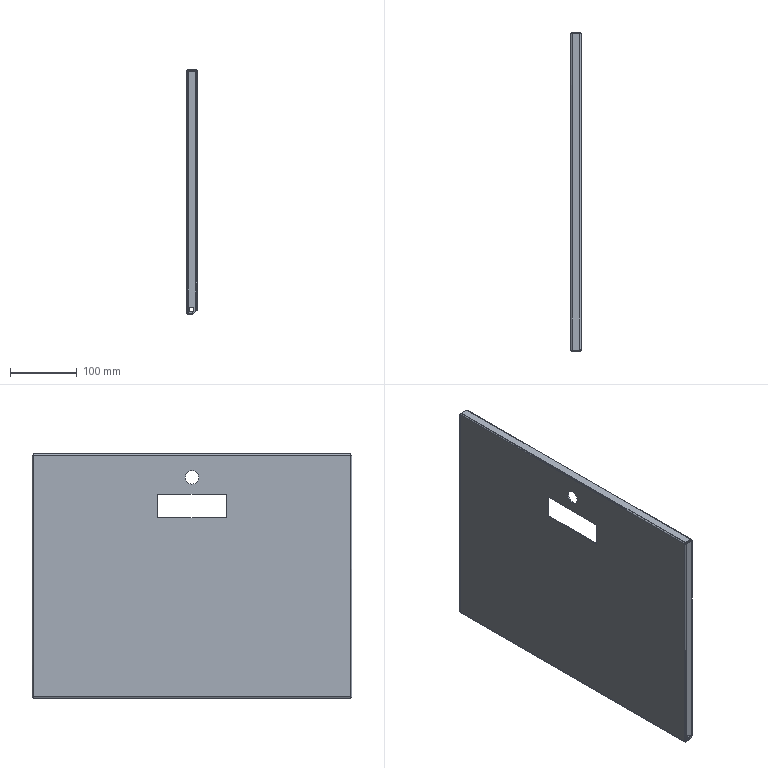Part | SolidWorks | features EdgeFlange 4, ICE 4, FlatPattern 1, SMBaseFlange 1, SheetMetal 1 | 1 solid | 92 faces | box 15 x 477 x 364.5 mm | volume 307164 mm3 | plane 62 | cylinder 22 | spline 8 | commonest cylinder face diameters 0.6 x7 3.6 x7 7 x4 20 x2 1.473 x1 4.473 x1